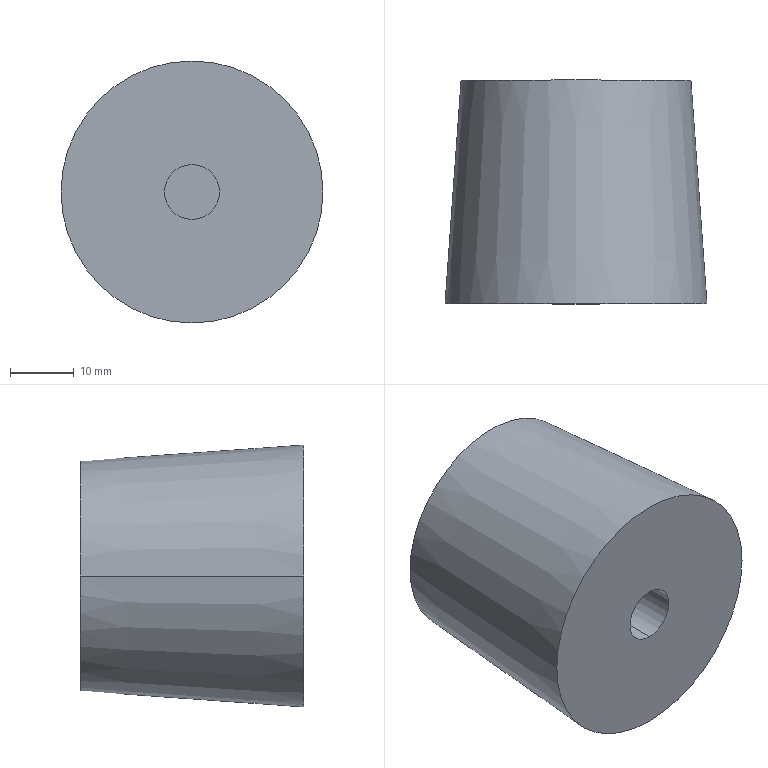Part | STEP file | SOLID | 1 solid | 10 faces | box 41 x 35 x 41 mm | volume 39118 mm3 | plane 4 | cylinder 4 | cone 2 | commonest cylinder face diameters 8.6 x4
STEP:
#1=CARTESIAN_POINT('',(0.,0.,0.));
#2=DIRECTION('',(0.,0.,1.));
#3=DIRECTION('',(1.,0.,0.));
#4=AXIS2_PLACEMENT_3D('',#1,#2,#3);
#5=CARTESIAN_POINT('',(20.5,0.,0.));
#6=VERTEX_POINT('',#5);
#7=CARTESIAN_POINT('',(-20.5,0.,0.));
#8=VERTEX_POINT('',#7);
#9=CARTESIAN_POINT('',(0.,0.,0.));
#10=DIRECTION('',(0.,1.,0.));
#11=DIRECTION('',(1.,0.,0.));
#12=AXIS2_PLACEMENT_3D('',#9,#10,#11);
#13=CIRCLE('',#12,20.5);
#14=CARTESIAN_POINT('',(0.,0.,0.));
#15=DIRECTION('',(0.,1.,0.));
#16=DIRECTION('',(1.,0.,0.));
#17=AXIS2_PLACEMENT_3D('',#14,#15,#16);
#18=PLANE('',#17);
#19=CARTESIAN_POINT('',(0.,0.));
#20=DIRECTION('',(1.,0.));
#21=AXIS2_PLACEMENT_2D('',#19,#20);
#22=CIRCLE('',#21,20.5);
#23=(GEOMETRIC_REPRESENTATION_CONTEXT(2)PARAMETRIC_REPRESENTATION_CONTEXT()REPRESENTATION_CONTEXT('',''));
#24=DEFINITIONAL_REPRESENTATION('',(#22),#23);
#25=PCURVE('',#18,#24);
#26=CARTESIAN_POINT('',(0.,17.5,0.));
#27=DIRECTION('',(0.,-1.,0.));
#28=DIRECTION('',(-1.,0.,0.));
#29=AXIS2_PLACEMENT_3D('',#26,#27,#28);
#30=CONICAL_SURFACE('',#29,19.25,0.07131);
#31=CARTESIAN_POINT('',(3.142,17.5));
#32=DIRECTION('',(-1.,0.));
#33=VECTOR('',#32,1.);
#34=LINE('',#31,#33);
#35=(GEOMETRIC_REPRESENTATION_CONTEXT(2)PARAMETRIC_REPRESENTATION_CONTEXT()REPRESENTATION_CONTEXT('',''));
#36=DEFINITIONAL_REPRESENTATION('',(#34),#35);
#37=PCURVE('',#30,#36);
#38=SURFACE_CURVE('',#13,(#25,#37),.PCURVE_S1.);
#39=EDGE_CURVE('',#6,#8,#38,.T.);
#40=ORIENTED_EDGE('',*,*,#39,.T.);
#41=CARTESIAN_POINT('',(0.,0.,0.));
#42=DIRECTION('',(0.,1.,0.));
#43=DIRECTION('',(-1.,0.,0.));
#44=AXIS2_PLACEMENT_3D('',#41,#42,#43);
#45=CIRCLE('',#44,20.5);
#46=CARTESIAN_POINT('',(0.,0.));
#47=DIRECTION('',(-1.,0.));
#48=AXIS2_PLACEMENT_2D('',#46,#47);
#49=CIRCLE('',#48,20.5);
#50=(GEOMETRIC_REPRESENTATION_CONTEXT(2)PARAMETRIC_REPRESENTATION_CONTEXT()REPRESENTATION_CONTEXT('',''));
#51=DEFINITIONAL_REPRESENTATION('',(#49),#50);
#52=PCURVE('',#18,#51);
#53=CARTESIAN_POINT('',(0.,17.5,0.));
#54=DIRECTION('',(0.,-1.,0.));
#55=DIRECTION('',(1.,0.,0.));
#56=AXIS2_PLACEMENT_3D('',#53,#54,#55);
#57=CONICAL_SURFACE('',#56,19.25,0.07131);
#58=CARTESIAN_POINT('',(3.142,17.5));
#59=DIRECTION('',(-1.,0.));
#60=VECTOR('',#59,1.);
#61=LINE('',#58,#60);
#62=(GEOMETRIC_REPRESENTATION_CONTEXT(2)PARAMETRIC_REPRESENTATION_CONTEXT()REPRESENTATION_CONTEXT('',''));
#63=DEFINITIONAL_REPRESENTATION('',(#61),#62);
#64=PCURVE('',#57,#63);
#65=SURFACE_CURVE('',#45,(#52,#64),.PCURVE_S1.);
#66=EDGE_CURVE('',#8,#6,#65,.T.);
#67=ORIENTED_EDGE('',*,*,#66,.T.);
#68=EDGE_LOOP('',(#40,#67));
#69=FACE_BOUND('',#68,.F.);
#70=CARTESIAN_POINT('',(0.,0.,-4.3));
#71=VERTEX_POINT('',#70);
#72=CARTESIAN_POINT('',(0.,0.,4.3));
#73=VERTEX_POINT('',#72);
#74=CARTESIAN_POINT('',(0.,0.,0.));
#75=DIRECTION('',(0.,-1.,0.));
#76=DIRECTION('',(0.,0.,-1.));
#77=AXIS2_PLACEMENT_3D('',#74,#75,#76);
#78=CIRCLE('',#77,4.3);
#79=CARTESIAN_POINT('',(0.,4.3));
#80=CARTESIAN_POINT('',(7.448,4.3));
#81=CARTESIAN_POINT('',(3.724,-2.15));
#82=CARTESIAN_POINT('',(0.,-8.6));
#83=CARTESIAN_POINT('',(-3.724,-2.15));
#84=CARTESIAN_POINT('',(-7.448,4.3));
#85=CARTESIAN_POINT('',(0.,4.3));
#86=(BOUNDED_CURVE()B_SPLINE_CURVE(2,(#79,#80,#81,#82,#83,#84,#85),.UNSPECIFIED.,.T.,.F.)B_SPLINE_CURVE_WITH_KNOTS((1,2,2,2,2,1),(-2.094,0.,2.094,4.189,6.283,8.378),.UNSPECIFIED.)CURVE()GEOMETRIC_REPRESENTATION_ITEM()RATIONAL_B_SPLINE_CURVE((1.,0.5,1.,0.5,1.,0.5,1.))REPRESENTATION_ITEM(''));
#87=(GEOMETRIC_REPRESENTATION_CONTEXT(2)PARAMETRIC_REPRESENTATION_CONTEXT()REPRESENTATION_CONTEXT('',''));
#88=DEFINITIONAL_REPRESENTATION('',(#86),#87);
#89=PCURVE('',#18,#88);
#90=CARTESIAN_POINT('',(0.,0.,0.));
#91=DIRECTION('',(0.,-1.,0.));
#92=DIRECTION('',(0.,0.,-1.));
#93=AXIS2_PLACEMENT_3D('',#90,#91,#92);
#94=CYLINDRICAL_SURFACE('',#93,4.3);
#95=CARTESIAN_POINT('',(0.,0.));
#96=DIRECTION('',(1.,0.));
#97=VECTOR('',#96,1.);
#98=LINE('',#95,#97);
#99=(GEOMETRIC_REPRESENTATION_CONTEXT(2)PARAMETRIC_REPRESENTATION_CONTEXT()REPRESENTATION_CONTEXT('',''));
#100=DEFINITIONAL_REPRESENTATION('',(#98),#99);
#101=PCURVE('',#94,#100);
#102=SURFACE_CURVE('',#78,(#89,#101),.PCURVE_S1.);
#103=EDGE_CURVE('',#71,#73,#102,.T.);
#104=ORIENTED_EDGE('',*,*,#103,.T.);
#105=CARTESIAN_POINT('',(0.,0.,0.));
#106=DIRECTION('',(0.,-1.,0.));
#107=DIRECTION('',(0.,0.,1.));
#108=AXIS2_PLACEMENT_3D('',#105,#106,#107);
#109=CIRCLE('',#108,4.3);
#110=CARTESIAN_POINT('',(0.,-4.3));
#111=CARTESIAN_POINT('',(-7.448,-4.3));
#112=CARTESIAN_POINT('',(-3.724,2.15));
#113=CARTESIAN_POINT('',(0.,8.6));
#114=CARTESIAN_POINT('',(3.724,2.15));
#115=CARTESIAN_POINT('',(7.448,-4.3));
#116=CARTESIAN_POINT('',(0.,-4.3));
#117=(BOUNDED_CURVE()B_SPLINE_CURVE(2,(#110,#111,#112,#113,#114,#115,#116),.UNSPECIFIED.,.T.,.F.)B_SPLINE_CURVE_WITH_KNOTS((1,2,2,2,2,1),(-2.094,0.,2.094,4.189,6.283,8.378),.UNSPECIFIED.)CURVE()GEOMETRIC_REPRESENTATION_ITEM()RATIONAL_B_SPLINE_CURVE((1.,0.5,1.,0.5,1.,0.5,1.))REPRESENTATION_ITEM(''));
#118=(GEOMETRIC_REPRESENTATION_CONTEXT(2)PARAMETRIC_REPRESENTATION_CONTEXT()REPRESENTATION_CONTEXT('',''));
#119=DEFINITIONAL_REPRESENTATION('',(#117),#118);
#120=PCURVE('',#18,#119);
#121=CARTESIAN_POINT('',(0.,0.,0.));
#122=DIRECTION('',(0.,-1.,0.));
#123=DIRECTION('',(0.,0.,-1.));
#124=AXIS2_PLACEMENT_3D('',#121,#122,#123);
#125=CYLINDRICAL_SURFACE('',#124,4.3);
#126=CARTESIAN_POINT('',(3.142,0.));
#127=DIRECTION('',(1.,0.));
#128=VECTOR('',#127,1.);
#129=LINE('',#126,#128);
#130=(GEOMETRIC_REPRESENTATION_CONTEXT(2)PARAMETRIC_REPRESENTATION_CONTEXT()REPRESENTATION_CONTEXT('',''));
#131=DEFINITIONAL_REPRESENTATION('',(#129),#130);
#132=PCURVE('',#125,#131);
#133=SURFACE_CURVE('',#109,(#120,#132),.PCURVE_S1.);
#134=EDGE_CURVE('',#73,#71,#133,.T.);
#135=ORIENTED_EDGE('',*,*,#134,.T.);
#136=EDGE_LOOP('',(#104,#135));
#137=FACE_BOUND('',#136,.F.);
#138=ADVANCED_FACE('',(#69,#137),#18,.F.);
#139=CARTESIAN_POINT('',(-18.,35.,0.));
#140=VERTEX_POINT('',#139);
#141=CARTESIAN_POINT('',(-20.5,0.,0.));
#142=DIRECTION('',(0.07125,0.9975,0.));
#143=VECTOR('',#142,1.);
#144=LINE('',#141,#143);
#145=CARTESIAN_POINT('',(0.,17.5));
#146=DIRECTION('',(0.,-1.));
#147=VECTOR('',#146,1.);
#148=LINE('',#145,#147);
#149=(GEOMETRIC_REPRESENTATION_CONTEXT(2)PARAMETRIC_REPRESENTATION_CONTEXT()REPRESENTATION_CONTEXT('',''));
#150=DEFINITIONAL_REPRESENTATION('',(#148),#149);
#151=PCURVE('',#30,#150);
#152=CARTESIAN_POINT('',(3.142,17.5));
#153=DIRECTION('',(0.,-1.));
#154=VECTOR('',#153,1.);
#155=LINE('',#152,#154);
#156=(GEOMETRIC_REPRESENTATION_CONTEXT(2)PARAMETRIC_REPRESENTATION_CONTEXT()REPRESENTATION_CONTEXT('',''));
#157=DEFINITIONAL_REPRESENTATION('',(#155),#156);
#158=PCURVE('',#57,#157);
#159=SURFACE_CURVE('',#144,(#151,#158),.PCURVE_S1.);
#160=EDGE_CURVE('',#8,#140,#159,.T.);
#161=ORIENTED_EDGE('',*,*,#160,.T.);
#162=CARTESIAN_POINT('',(18.,35.,0.));
#163=VERTEX_POINT('',#162);
#164=CARTESIAN_POINT('',(0.,35.,0.));
#165=DIRECTION('',(0.,1.,0.));
#166=DIRECTION('',(1.,0.,0.));
#167=AXIS2_PLACEMENT_3D('',#164,#165,#166);
#168=CIRCLE('',#167,18.);
#169=CARTESIAN_POINT('',(3.142,-17.5));
#170=DIRECTION('',(-1.,0.));
#171=VECTOR('',#170,1.);
#172=LINE('',#169,#171);
#173=(GEOMETRIC_REPRESENTATION_CONTEXT(2)PARAMETRIC_REPRESENTATION_CONTEXT()REPRESENTATION_CONTEXT('',''));
#174=DEFINITIONAL_REPRESENTATION('',(#172),#173);
#175=PCURVE('',#30,#174);
#176=CARTESIAN_POINT('',(0.,35.,0.));
#177=DIRECTION('',(0.,1.,0.));
#178=DIRECTION('',(1.,0.,0.));
#179=AXIS2_PLACEMENT_3D('',#176,#177,#178);
#180=PLANE('',#179);
#181=CARTESIAN_POINT('',(0.,0.));
#182=DIRECTION('',(1.,0.));
#183=AXIS2_PLACEMENT_2D('',#181,#182);
#184=CIRCLE('',#183,18.);
#185=(GEOMETRIC_REPRESENTATION_CONTEXT(2)PARAMETRIC_REPRESENTATION_CONTEXT()REPRESENTATION_CONTEXT('',''));
#186=DEFINITIONAL_REPRESENTATION('',(#184),#185);
#187=PCURVE('',#180,#186);
#188=SURFACE_CURVE('',#168,(#175,#187),.PCURVE_S1.);
#189=EDGE_CURVE('',#163,#140,#188,.T.);
#190=ORIENTED_EDGE('',*,*,#189,.F.);
#191=CARTESIAN_POINT('',(20.5,0.,0.));
#192=DIRECTION('',(-0.07125,0.9975,0.));
#193=VECTOR('',#192,1.);
#194=LINE('',#191,#193);
#195=CARTESIAN_POINT('',(3.142,17.5));
#196=DIRECTION('',(0.,-1.));
#197=VECTOR('',#196,1.);
#198=LINE('',#195,#197);
#199=(GEOMETRIC_REPRESENTATION_CONTEXT(2)PARAMETRIC_REPRESENTATION_CONTEXT()REPRESENTATION_CONTEXT('',''));
#200=DEFINITIONAL_REPRESENTATION('',(#198),#199);
#201=PCURVE('',#30,#200);
#202=CARTESIAN_POINT('',(0.,17.5));
#203=DIRECTION('',(0.,-1.));
#204=VECTOR('',#203,1.);
#205=LINE('',#202,#204);
#206=(GEOMETRIC_REPRESENTATION_CONTEXT(2)PARAMETRIC_REPRESENTATION_CONTEXT()REPRESENTATION_CONTEXT('',''));
#207=DEFINITIONAL_REPRESENTATION('',(#205),#206);
#208=PCURVE('',#57,#207);
#209=SURFACE_CURVE('',#194,(#201,#208),.PCURVE_S1.);
#210=EDGE_CURVE('',#6,#163,#209,.T.);
#211=ORIENTED_EDGE('',*,*,#210,.F.);
#212=ORIENTED_EDGE('',*,*,#39,.T.);
#213=EDGE_LOOP('',(#161,#190,#211,#212));
#214=FACE_BOUND('',#213,.T.);
#215=ADVANCED_FACE('',(#214),#30,.T.);
#216=ORIENTED_EDGE('',*,*,#210,.T.);
#217=CARTESIAN_POINT('',(0.,35.,0.));
#218=DIRECTION('',(0.,1.,0.));
#219=DIRECTION('',(-1.,0.,0.));
#220=AXIS2_PLACEMENT_3D('',#217,#218,#219);
#221=CIRCLE('',#220,18.);
#222=CARTESIAN_POINT('',(3.142,-17.5));
#223=DIRECTION('',(-1.,0.));
#224=VECTOR('',#223,1.);
#225=LINE('',#222,#224);
#226=(GEOMETRIC_REPRESENTATION_CONTEXT(2)PARAMETRIC_REPRESENTATION_CONTEXT()REPRESENTATION_CONTEXT('',''));
#227=DEFINITIONAL_REPRESENTATION('',(#225),#226);
#228=PCURVE('',#57,#227);
#229=CARTESIAN_POINT('',(0.,0.));
#230=DIRECTION('',(-1.,0.));
#231=AXIS2_PLACEMENT_2D('',#229,#230);
#232=CIRCLE('',#231,18.);
#233=(GEOMETRIC_REPRESENTATION_CONTEXT(2)PARAMETRIC_REPRESENTATION_CONTEXT()REPRESENTATION_CONTEXT('',''));
#234=DEFINITIONAL_REPRESENTATION('',(#232),#233);
#235=PCURVE('',#180,#234);
#236=SURFACE_CURVE('',#221,(#228,#235),.PCURVE_S1.);
#237=EDGE_CURVE('',#140,#163,#236,.T.);
#238=ORIENTED_EDGE('',*,*,#237,.F.);
#239=ORIENTED_EDGE('',*,*,#160,.F.);
#240=ORIENTED_EDGE('',*,*,#66,.T.);
#241=EDGE_LOOP('',(#216,#238,#239,#240));
#242=FACE_BOUND('',#241,.T.);
#243=ADVANCED_FACE('',(#242),#57,.T.);
#244=ORIENTED_EDGE('',*,*,#189,.F.);
#245=ORIENTED_EDGE('',*,*,#237,.F.);
#246=EDGE_LOOP('',(#244,#245));
#247=FACE_BOUND('',#246,.F.);
#248=CARTESIAN_POINT('',(-4.3,35.,0.));
#249=VERTEX_POINT('',#248);
#250=CARTESIAN_POINT('',(4.3,35.,0.));
#251=VERTEX_POINT('',#250);
#252=CARTESIAN_POINT('',(0.,35.,0.));
#253=DIRECTION('',(0.,1.,0.));
#254=DIRECTION('',(-1.,0.,0.));
#255=AXIS2_PLACEMENT_3D('',#252,#253,#254);
#256=CIRCLE('',#255,4.3);
#257=CARTESIAN_POINT('',(0.,0.));
#258=DIRECTION('',(-1.,0.));
#259=AXIS2_PLACEMENT_2D('',#257,#258);
#260=CIRCLE('',#259,4.3);
#261=(GEOMETRIC_REPRESENTATION_CONTEXT(2)PARAMETRIC_REPRESENTATION_CONTEXT()REPRESENTATION_CONTEXT('',''));
#262=DEFINITIONAL_REPRESENTATION('',(#260),#261);
#263=PCURVE('',#180,#262);
#264=CARTESIAN_POINT('',(0.,35.,0.));
#265=DIRECTION('',(0.,1.,0.));
#266=DIRECTION('',(-1.,0.,0.));
#267=AXIS2_PLACEMENT_3D('',#264,#265,#266);
#268=CYLINDRICAL_SURFACE('',#267,4.3);
#269=CARTESIAN_POINT('',(0.,0.));
#270=DIRECTION('',(1.,0.));
#271=VECTOR('',#270,1.);
#272=LINE('',#269,#271);
#273=(GEOMETRIC_REPRESENTATION_CONTEXT(2)PARAMETRIC_REPRESENTATION_CONTEXT()REPRESENTATION_CONTEXT('',''));
#274=DEFINITIONAL_REPRESENTATION('',(#272),#273);
#275=PCURVE('',#268,#274);
#276=SURFACE_CURVE('',#256,(#263,#275),.PCURVE_S1.);
#277=EDGE_CURVE('',#249,#251,#276,.T.);
#278=ORIENTED_EDGE('',*,*,#277,.T.);
#279=CARTESIAN_POINT('',(0.,35.,0.));
#280=DIRECTION('',(0.,1.,0.));
#281=DIRECTION('',(1.,0.,0.));
#282=AXIS2_PLACEMENT_3D('',#279,#280,#281);
#283=CIRCLE('',#282,4.3);
#284=CARTESIAN_POINT('',(0.,0.));
#285=DIRECTION('',(1.,0.));
#286=AXIS2_PLACEMENT_2D('',#284,#285);
#287=CIRCLE('',#286,4.3);
#288=(GEOMETRIC_REPRESENTATION_CONTEXT(2)PARAMETRIC_REPRESENTATION_CONTEXT()REPRESENTATION_CONTEXT('',''));
#289=DEFINITIONAL_REPRESENTATION('',(#287),#288);
#290=PCURVE('',#180,#289);
#291=CARTESIAN_POINT('',(0.,35.,0.));
#292=DIRECTION('',(0.,1.,0.));
#293=DIRECTION('',(-1.,0.,0.));
#294=AXIS2_PLACEMENT_3D('',#291,#292,#293);
#295=CYLINDRICAL_SURFACE('',#294,4.3);
#296=CARTESIAN_POINT('',(3.142,0.));
#297=DIRECTION('',(1.,0.));
#298=VECTOR('',#297,1.);
#299=LINE('',#296,#298);
#300=(GEOMETRIC_REPRESENTATION_CONTEXT(2)PARAMETRIC_REPRESENTATION_CONTEXT()REPRESENTATION_CONTEXT('',''));
#301=DEFINITIONAL_REPRESENTATION('',(#299),#300);
#302=PCURVE('',#295,#301);
#303=SURFACE_CURVE('',#283,(#290,#302),.PCURVE_S1.);
#304=EDGE_CURVE('',#251,#249,#303,.T.);
#305=ORIENTED_EDGE('',*,*,#304,.T.);
#306=EDGE_LOOP('',(#278,#305));
#307=FACE_BOUND('',#306,.F.);
#308=ADVANCED_FACE('',(#247,#307),#180,.T.);
#309=ORIENTED_EDGE('',*,*,#277,.F.);
#310=CARTESIAN_POINT('',(-4.3,20.5,0.));
#311=VERTEX_POINT('',#310);
#312=CARTESIAN_POINT('',(-4.3,35.,0.));
#313=DIRECTION('',(0.,-1.,0.));
#314=VECTOR('',#313,1.);
#315=LINE('',#312,#314);
#316=CARTESIAN_POINT('',(0.,0.));
#317=DIRECTION('',(0.,-1.));
#318=VECTOR('',#317,1.);
#319=LINE('',#316,#318);
#320=(GEOMETRIC_REPRESENTATION_CONTEXT(2)PARAMETRIC_REPRESENTATION_CONTEXT()REPRESENTATION_CONTEXT('',''));
#321=DEFINITIONAL_REPRESENTATION('',(#319),#320);
#322=PCURVE('',#268,#321);
#323=CARTESIAN_POINT('',(6.283,0.));
#324=DIRECTION('',(0.,-1.));
#325=VECTOR('',#324,1.);
#326=LINE('',#323,#325);
#327=(GEOMETRIC_REPRESENTATION_CONTEXT(2)PARAMETRIC_REPRESENTATION_CONTEXT()REPRESENTATION_CONTEXT('',''));
#328=DEFINITIONAL_REPRESENTATION('',(#326),#327);
#329=PCURVE('',#295,#328);
#330=SURFACE_CURVE('',#315,(#322,#329),.PCURVE_S1.);
#331=EDGE_CURVE('',#249,#311,#330,.T.);
#332=ORIENTED_EDGE('',*,*,#331,.T.);
#333=CARTESIAN_POINT('',(4.3,20.5,0.));
#334=VERTEX_POINT('',#333);
#335=CARTESIAN_POINT('',(0.,20.5,0.));
#336=DIRECTION('',(0.,1.,0.));
#337=DIRECTION('',(-1.,0.,0.));
#338=AXIS2_PLACEMENT_3D('',#335,#336,#337);
#339=CIRCLE('',#338,4.3);
#340=CARTESIAN_POINT('',(0.,-14.5));
#341=DIRECTION('',(1.,0.));
#342=VECTOR('',#341,1.);
#343=LINE('',#340,#342);
#344=(GEOMETRIC_REPRESENTATION_CONTEXT(2)PARAMETRIC_REPRESENTATION_CONTEXT()REPRESENTATION_CONTEXT('',''));
#345=DEFINITIONAL_REPRESENTATION('',(#343),#344);
#346=PCURVE('',#268,#345);
#347=CARTESIAN_POINT('',(0.,20.5,0.));
#348=DIRECTION('',(0.,1.,0.));
#349=DIRECTION('',(-1.,0.,0.));
#350=AXIS2_PLACEMENT_3D('',#347,#348,#349);
#351=PLANE('',#350);
#352=CARTESIAN_POINT('',(0.,0.));
#353=DIRECTION('',(1.,0.));
#354=AXIS2_PLACEMENT_2D('',#352,#353);
#355=CIRCLE('',#354,4.3);
#356=(GEOMETRIC_REPRESENTATION_CONTEXT(2)PARAMETRIC_REPRESENTATION_CONTEXT()REPRESENTATION_CONTEXT('',''));
#357=DEFINITIONAL_REPRESENTATION('',(#355),#356);
#358=PCURVE('',#351,#357);
#359=SURFACE_CURVE('',#339,(#346,#358),.PCURVE_S1.);
#360=EDGE_CURVE('',#311,#334,#359,.T.);
#361=ORIENTED_EDGE('',*,*,#360,.T.);
#362=CARTESIAN_POINT('',(4.3,35.,0.));
#363=DIRECTION('',(0.,-1.,0.));
#364=VECTOR('',#363,1.);
#365=LINE('',#362,#364);
#366=CARTESIAN_POINT('',(3.142,0.));
#367=DIRECTION('',(0.,-1.));
#368=VECTOR('',#367,1.);
#369=LINE('',#366,#368);
#370=(GEOMETRIC_REPRESENTATION_CONTEXT(2)PARAMETRIC_REPRESENTATION_CONTEXT()REPRESENTATION_CONTEXT('',''));
#371=DEFINITIONAL_REPRESENTATION('',(#369),#370);
#372=PCURVE('',#268,#371);
#373=CARTESIAN_POINT('',(3.142,0.));
#374=DIRECTION('',(0.,-1.));
#375=VECTOR('',#374,1.);
#376=LINE('',#373,#375);
#377=(GEOMETRIC_REPRESENTATION_CONTEXT(2)PARAMETRIC_REPRESENTATION_CONTEXT()REPRESENTATION_CONTEXT('',''));
#378=DEFINITIONAL_REPRESENTATION('',(#376),#377);
#379=PCURVE('',#295,#378);
#380=SURFACE_CURVE('',#365,(#372,#379),.PCURVE_S1.);
#381=EDGE_CURVE('',#251,#334,#380,.T.);
#382=ORIENTED_EDGE('',*,*,#381,.F.);
#383=EDGE_LOOP('',(#309,#332,#361,#382));
#384=FACE_BOUND('',#383,.F.);
#385=ADVANCED_FACE('',(#384),#268,.F.);
#386=ORIENTED_EDGE('',*,*,#304,.F.);
#387=ORIENTED_EDGE('',*,*,#381,.T.);
#388=CARTESIAN_POINT('',(0.,20.5,0.));
#389=DIRECTION('',(0.,1.,0.));
#390=DIRECTION('',(1.,0.,0.));
#391=AXIS2_PLACEMENT_3D('',#388,#389,#390);
#392=CIRCLE('',#391,4.3);
#393=CARTESIAN_POINT('',(3.142,-14.5));
#394=DIRECTION('',(1.,0.));
#395=VECTOR('',#394,1.);
#396=LINE('',#393,#395);
#397=(GEOMETRIC_REPRESENTATION_CONTEXT(2)PARAMETRIC_REPRESENTATION_CONTEXT()REPRESENTATION_CONTEXT('',''));
#398=DEFINITIONAL_REPRESENTATION('',(#396),#397);
#399=PCURVE('',#295,#398);
#400=CARTESIAN_POINT('',(0.,0.));
#401=DIRECTION('',(-1.,0.));
#402=AXIS2_PLACEMENT_2D('',#400,#401);
#403=CIRCLE('',#402,4.3);
#404=(GEOMETRIC_REPRESENTATION_CONTEXT(2)PARAMETRIC_REPRESENTATION_CONTEXT()REPRESENTATION_CONTEXT('',''));
#405=DEFINITIONAL_REPRESENTATION('',(#403),#404);
#406=PCURVE('',#351,#405);
#407=SURFACE_CURVE('',#392,(#399,#406),.PCURVE_S1.);
#408=EDGE_CURVE('',#334,#311,#407,.T.);
#409=ORIENTED_EDGE('',*,*,#408,.T.);
#410=ORIENTED_EDGE('',*,*,#331,.F.);
#411=EDGE_LOOP('',(#386,#387,#409,#410));
#412=FACE_BOUND('',#411,.F.);
#413=ADVANCED_FACE('',(#412),#295,.F.);
#414=ORIENTED_EDGE('',*,*,#360,.F.);
#415=ORIENTED_EDGE('',*,*,#408,.F.);
#416=EDGE_LOOP('',(#414,#415));
#417=FACE_BOUND('',#416,.F.);
#418=ADVANCED_FACE('',(#417),#351,.T.);
#419=ORIENTED_EDGE('',*,*,#103,.F.);
#420=CARTESIAN_POINT('',(0.,14.5,-4.3));
#421=VERTEX_POINT('',#420);
#422=CARTESIAN_POINT('',(0.,0.,-4.3));
#423=DIRECTION('',(0.,1.,0.));
#424=VECTOR('',#423,1.);
#425=LINE('',#422,#424);
#426=CARTESIAN_POINT('',(0.,0.));
#427=DIRECTION('',(0.,-1.));
#428=VECTOR('',#427,1.);
#429=LINE('',#426,#428);
#430=(GEOMETRIC_REPRESENTATION_CONTEXT(2)PARAMETRIC_REPRESENTATION_CONTEXT()REPRESENTATION_CONTEXT('',''));
#431=DEFINITIONAL_REPRESENTATION('',(#429),#430);
#432=PCURVE('',#94,#431);
#433=CARTESIAN_POINT('',(6.283,0.));
#434=DIRECTION('',(0.,-1.));
#435=VECTOR('',#434,1.);
#436=LINE('',#433,#435);
#437=(GEOMETRIC_REPRESENTATION_CONTEXT(2)PARAMETRIC_REPRESENTATION_CONTEXT()REPRESENTATION_CONTEXT('',''));
#438=DEFINITIONAL_REPRESENTATION('',(#436),#437);
#439=PCURVE('',#125,#438);
#440=SURFACE_CURVE('',#425,(#432,#439),.PCURVE_S1.);
#441=EDGE_CURVE('',#71,#421,#440,.T.);
#442=ORIENTED_EDGE('',*,*,#441,.T.);
#443=CARTESIAN_POINT('',(0.,14.5,4.3));
#444=VERTEX_POINT('',#443);
#445=CARTESIAN_POINT('',(0.,14.5,0.));
#446=DIRECTION('',(0.,-1.,0.));
#447=DIRECTION('',(0.,0.,-1.));
#448=AXIS2_PLACEMENT_3D('',#445,#446,#447);
#449=CIRCLE('',#448,4.3);
#450=CARTESIAN_POINT('',(0.,-14.5));
#451=DIRECTION('',(1.,0.));
#452=VECTOR('',#451,1.);
#453=LINE('',#450,#452);
#454=(GEOMETRIC_REPRESENTATION_CONTEXT(2)PARAMETRIC_REPRESENTATION_CONTEXT()REPRESENTATION_CONTEXT('',''));
#455=DEFINITIONAL_REPRESENTATION('',(#453),#454);
#456=PCURVE('',#94,#455);
#457=CARTESIAN_POINT('',(0.,14.5,0.));
#458=DIRECTION('',(0.,-1.,0.));
#459=DIRECTION('',(0.,0.,-1.));
#460=AXIS2_PLACEMENT_3D('',#457,#458,#459);
#461=PLANE('',#460);
#462=CARTESIAN_POINT('',(0.,0.));
#463=DIRECTION('',(1.,0.));
#464=AXIS2_PLACEMENT_2D('',#462,#463);
#465=CIRCLE('',#464,4.3);
#466=(GEOMETRIC_REPRESENTATION_CONTEXT(2)PARAMETRIC_REPRESENTATION_CONTEXT()REPRESENTATION_CONTEXT('',''));
#467=DEFINITIONAL_REPRESENTATION('',(#465),#466);
#468=PCURVE('',#461,#467);
#469=SURFACE_CURVE('',#449,(#456,#468),.PCURVE_S1.);
#470=EDGE_CURVE('',#421,#444,#469,.T.);
#471=ORIENTED_EDGE('',*,*,#470,.T.);
#472=CARTESIAN_POINT('',(0.,0.,4.3));
#473=DIRECTION('',(0.,1.,0.));
#474=VECTOR('',#473,1.);
#475=LINE('',#472,#474);
#476=CARTESIAN_POINT('',(3.142,0.));
#477=DIRECTION('',(0.,-1.));
#478=VECTOR('',#477,1.);
#479=LINE('',#476,#478);
#480=(GEOMETRIC_REPRESENTATION_CONTEXT(2)PARAMETRIC_REPRESENTATION_CONTEXT()REPRESENTATION_CONTEXT('',''));
#481=DEFINITIONAL_REPRESENTATION('',(#479),#480);
#482=PCURVE('',#94,#481);
#483=CARTESIAN_POINT('',(3.142,0.));
#484=DIRECTION('',(0.,-1.));
#485=VECTOR('',#484,1.);
#486=LINE('',#483,#485);
#487=(GEOMETRIC_REPRESENTATION_CONTEXT(2)PARAMETRIC_REPRESENTATION_CONTEXT()REPRESENTATION_CONTEXT('',''));
#488=DEFINITIONAL_REPRESENTATION('',(#486),#487);
#489=PCURVE('',#125,#488);
#490=SURFACE_CURVE('',#475,(#482,#489),.PCURVE_S1.);
#491=EDGE_CURVE('',#73,#444,#490,.T.);
#492=ORIENTED_EDGE('',*,*,#491,.F.);
#493=EDGE_LOOP('',(#419,#442,#471,#492));
#494=FACE_BOUND('',#493,.F.);
#495=ADVANCED_FACE('',(#494),#94,.F.);
#496=ORIENTED_EDGE('',*,*,#134,.F.);
#497=ORIENTED_EDGE('',*,*,#491,.T.);
#498=CARTESIAN_POINT('',(0.,14.5,0.));
#499=DIRECTION('',(0.,-1.,0.));
#500=DIRECTION('',(0.,0.,1.));
#501=AXIS2_PLACEMENT_3D('',#498,#499,#500);
#502=CIRCLE('',#501,4.3);
#503=CARTESIAN_POINT('',(3.142,-14.5));
#504=DIRECTION('',(1.,0.));
#505=VECTOR('',#504,1.);
#506=LINE('',#503,#505);
#507=(GEOMETRIC_REPRESENTATION_CONTEXT(2)PARAMETRIC_REPRESENTATION_CONTEXT()REPRESENTATION_CONTEXT('',''));
#508=DEFINITIONAL_REPRESENTATION('',(#506),#507);
#509=PCURVE('',#125,#508);
#510=CARTESIAN_POINT('',(0.,0.));
#511=DIRECTION('',(-1.,0.));
#512=AXIS2_PLACEMENT_2D('',#510,#511);
#513=CIRCLE('',#512,4.3);
#514=(GEOMETRIC_REPRESENTATION_CONTEXT(2)PARAMETRIC_REPRESENTATION_CONTEXT()REPRESENTATION_CONTEXT('',''));
#515=DEFINITIONAL_REPRESENTATION('',(#513),#514);
#516=PCURVE('',#461,#515);
#517=SURFACE_CURVE('',#502,(#509,#516),.PCURVE_S1.);
#518=EDGE_CURVE('',#444,#421,#517,.T.);
#519=ORIENTED_EDGE('',*,*,#518,.T.);
#520=ORIENTED_EDGE('',*,*,#441,.F.);
#521=EDGE_LOOP('',(#496,#497,#519,#520));
#522=FACE_BOUND('',#521,.F.);
#523=ADVANCED_FACE('',(#522),#125,.F.);
#524=ORIENTED_EDGE('',*,*,#470,.F.);
#525=ORIENTED_EDGE('',*,*,#518,.F.);
#526=EDGE_LOOP('',(#524,#525));
#527=FACE_BOUND('',#526,.F.);
#528=ADVANCED_FACE('',(#527),#461,.T.);
#529=CLOSED_SHELL('',(#138,#215,#243,#308,#385,#413,#418,#495,#523,#528));
#530=MANIFOLD_SOLID_BREP('',#529);
#531=(LENGTH_UNIT()NAMED_UNIT(*)SI_UNIT(.MILLI.,.METRE.));
#532=UNCERTAINTY_MEASURE_WITH_UNIT(LENGTH_MEASURE(0.0000001),#531,'','');
#533=(NAMED_UNIT(*)PLANE_ANGLE_UNIT()SI_UNIT($,.RADIAN.));
#534=(NAMED_UNIT(*)SI_UNIT($,.STERADIAN.)SOLID_ANGLE_UNIT());
#535=(GEOMETRIC_REPRESENTATION_CONTEXT(3)GLOBAL_UNCERTAINTY_ASSIGNED_CONTEXT((#532))GLOBAL_UNIT_ASSIGNED_CONTEXT((#531,#533,#534))REPRESENTATION_CONTEXT('',''));
#536=ADVANCED_BREP_SHAPE_REPRESENTATION('',(#4,#530),#535);